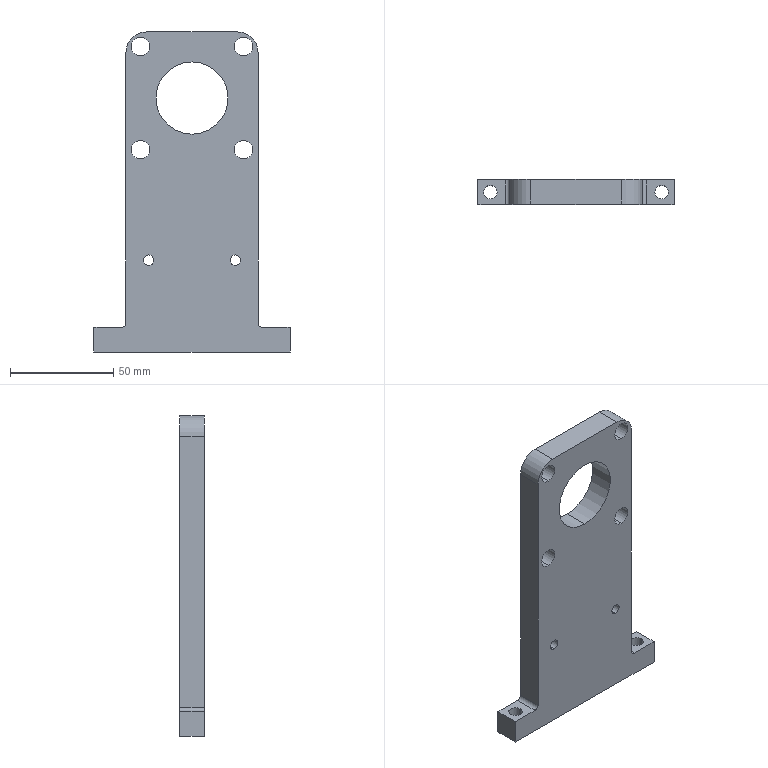Part | 1 solid | 40 faces | box 95 x 12 x 155 mm | volume 106731 mm3 | cylinder 26 | plane 10 | cone 4 | commonest cylinder face diameters 5 x8 9 x8 6.5 x4 4 x2 20 x2 35 x2
STEP:
#1=CARTESIAN_POINT('',(72.5,12.,102.5));
#2=VERTEX_POINT('',#1);
#3=CARTESIAN_POINT('',(72.5,12.,93.5));
#4=VERTEX_POINT('',#3);
#5=CARTESIAN_POINT('',(72.5,12.,98.));
#6=DIRECTION('',(0.,-1.,0.));
#7=DIRECTION('',(0.,0.,-1.));
#8=AXIS2_PLACEMENT_3D('',#5,#6,#7);
#9=CIRCLE('',#8,4.5);
#10=EDGE_CURVE('',#2,#4,#9,.T.);
#11=ORIENTED_EDGE('',*,*,#10,.F.);
#12=CARTESIAN_POINT('',(72.5,0.,102.5));
#13=VERTEX_POINT('',#12);
#14=CARTESIAN_POINT('',(72.5,0.,102.5));
#15=DIRECTION('',(0.,-1.,0.));
#16=VECTOR('',#15,1000.);
#17=LINE('',#14,#16);
#18=EDGE_CURVE('',#2,#13,#17,.T.);
#19=ORIENTED_EDGE('',*,*,#18,.T.);
#20=CARTESIAN_POINT('',(72.5,0.,93.5));
#21=VERTEX_POINT('',#20);
#22=CARTESIAN_POINT('',(72.5,0.,98.));
#23=DIRECTION('',(0.,-1.,0.));
#24=DIRECTION('',(0.,0.,-1.));
#25=AXIS2_PLACEMENT_3D('',#22,#23,#24);
#26=CIRCLE('',#25,4.5);
#27=EDGE_CURVE('',#13,#21,#26,.T.);
#28=ORIENTED_EDGE('',*,*,#27,.T.);
#29=CARTESIAN_POINT('',(72.5,0.,93.5));
#30=DIRECTION('',(0.,-1.,0.));
#31=VECTOR('',#30,1000.);
#32=LINE('',#29,#31);
#33=EDGE_CURVE('',#4,#21,#32,.T.);
#34=ORIENTED_EDGE('',*,*,#33,.F.);
#35=EDGE_LOOP('',(#11,#19,#28,#34));
#36=FACE_OUTER_BOUND('',#35,.T.);
#37=CARTESIAN_POINT('',(72.5,0.,98.));
#38=DIRECTION('',(0.,-1.,0.));
#39=DIRECTION('',(0.,0.,-1.));
#40=AXIS2_PLACEMENT_3D('',#37,#38,#39);
#41=CYLINDRICAL_SURFACE('',#40,4.5);
#42=ADVANCED_FACE('',(#36),#41,.F.);
#43=CARTESIAN_POINT('',(72.5,12.,152.5));
#44=VERTEX_POINT('',#43);
#45=CARTESIAN_POINT('',(72.5,12.,143.5));
#46=VERTEX_POINT('',#45);
#47=CARTESIAN_POINT('',(72.5,12.,148.));
#48=DIRECTION('',(0.,-1.,0.));
#49=DIRECTION('',(0.,0.,-1.));
#50=AXIS2_PLACEMENT_3D('',#47,#48,#49);
#51=CIRCLE('',#50,4.5);
#52=EDGE_CURVE('',#44,#46,#51,.T.);
#53=ORIENTED_EDGE('',*,*,#52,.F.);
#54=CARTESIAN_POINT('',(72.5,0.,152.5));
#55=VERTEX_POINT('',#54);
#56=CARTESIAN_POINT('',(72.5,0.,152.5));
#57=DIRECTION('',(0.,-1.,0.));
#58=VECTOR('',#57,1000.);
#59=LINE('',#56,#58);
#60=EDGE_CURVE('',#44,#55,#59,.T.);
#61=ORIENTED_EDGE('',*,*,#60,.T.);
#62=CARTESIAN_POINT('',(72.5,0.,143.5));
#63=VERTEX_POINT('',#62);
#64=CARTESIAN_POINT('',(72.5,0.,148.));
#65=DIRECTION('',(0.,-1.,0.));
#66=DIRECTION('',(0.,0.,-1.));
#67=AXIS2_PLACEMENT_3D('',#64,#65,#66);
#68=CIRCLE('',#67,4.5);
#69=EDGE_CURVE('',#55,#63,#68,.T.);
#70=ORIENTED_EDGE('',*,*,#69,.T.);
#71=CARTESIAN_POINT('',(72.5,0.,143.5));
#72=DIRECTION('',(0.,-1.,0.));
#73=VECTOR('',#72,1000.);
#74=LINE('',#71,#73);
#75=EDGE_CURVE('',#46,#63,#74,.T.);
#76=ORIENTED_EDGE('',*,*,#75,.F.);
#77=EDGE_LOOP('',(#53,#61,#70,#76));
#78=FACE_OUTER_BOUND('',#77,.T.);
#79=CARTESIAN_POINT('',(72.5,0.,148.));
#80=DIRECTION('',(0.,-1.,0.));
#81=DIRECTION('',(0.,0.,-1.));
#82=AXIS2_PLACEMENT_3D('',#79,#80,#81);
#83=CYLINDRICAL_SURFACE('',#82,4.5);
#84=ADVANCED_FACE('',(#78),#83,.F.);
#85=CARTESIAN_POINT('',(22.5,12.,152.5));
#86=VERTEX_POINT('',#85);
#87=CARTESIAN_POINT('',(22.5,12.,143.5));
#88=VERTEX_POINT('',#87);
#89=CARTESIAN_POINT('',(22.5,12.,148.));
#90=DIRECTION('',(0.,-1.,0.));
#91=DIRECTION('',(0.,0.,-1.));
#92=AXIS2_PLACEMENT_3D('',#89,#90,#91);
#93=CIRCLE('',#92,4.5);
#94=EDGE_CURVE('',#86,#88,#93,.T.);
#95=ORIENTED_EDGE('',*,*,#94,.F.);
#96=CARTESIAN_POINT('',(22.5,0.,152.5));
#97=VERTEX_POINT('',#96);
#98=CARTESIAN_POINT('',(22.5,0.,152.5));
#99=DIRECTION('',(0.,-1.,0.));
#100=VECTOR('',#99,1000.);
#101=LINE('',#98,#100);
#102=EDGE_CURVE('',#86,#97,#101,.T.);
#103=ORIENTED_EDGE('',*,*,#102,.T.);
#104=CARTESIAN_POINT('',(22.5,0.,143.5));
#105=VERTEX_POINT('',#104);
#106=CARTESIAN_POINT('',(22.5,0.,148.));
#107=DIRECTION('',(0.,-1.,0.));
#108=DIRECTION('',(0.,0.,-1.));
#109=AXIS2_PLACEMENT_3D('',#106,#107,#108);
#110=CIRCLE('',#109,4.5);
#111=EDGE_CURVE('',#97,#105,#110,.T.);
#112=ORIENTED_EDGE('',*,*,#111,.T.);
#113=CARTESIAN_POINT('',(22.5,0.,143.5));
#114=DIRECTION('',(0.,-1.,0.));
#115=VECTOR('',#114,1000.);
#116=LINE('',#113,#115);
#117=EDGE_CURVE('',#88,#105,#116,.T.);
#118=ORIENTED_EDGE('',*,*,#117,.F.);
#119=EDGE_LOOP('',(#95,#103,#112,#118));
#120=FACE_OUTER_BOUND('',#119,.T.);
#121=CARTESIAN_POINT('',(22.5,0.,148.));
#122=DIRECTION('',(0.,-1.,0.));
#123=DIRECTION('',(0.,0.,-1.));
#124=AXIS2_PLACEMENT_3D('',#121,#122,#123);
#125=CYLINDRICAL_SURFACE('',#124,4.5);
#126=ADVANCED_FACE('',(#120),#125,.F.);
#127=CARTESIAN_POINT('',(22.5,12.,102.5));
#128=VERTEX_POINT('',#127);
#129=CARTESIAN_POINT('',(22.5,12.,93.5));
#130=VERTEX_POINT('',#129);
#131=CARTESIAN_POINT('',(22.5,12.,98.));
#132=DIRECTION('',(0.,-1.,0.));
#133=DIRECTION('',(0.,0.,-1.));
#134=AXIS2_PLACEMENT_3D('',#131,#132,#133);
#135=CIRCLE('',#134,4.5);
#136=EDGE_CURVE('',#128,#130,#135,.T.);
#137=ORIENTED_EDGE('',*,*,#136,.F.);
#138=CARTESIAN_POINT('',(22.5,0.,102.5));
#139=VERTEX_POINT('',#138);
#140=CARTESIAN_POINT('',(22.5,0.,102.5));
#141=DIRECTION('',(0.,-1.,0.));
#142=VECTOR('',#141,1000.);
#143=LINE('',#140,#142);
#144=EDGE_CURVE('',#128,#139,#143,.T.);
#145=ORIENTED_EDGE('',*,*,#144,.T.);
#146=CARTESIAN_POINT('',(22.5,0.,93.5));
#147=VERTEX_POINT('',#146);
#148=CARTESIAN_POINT('',(22.5,0.,98.));
#149=DIRECTION('',(0.,-1.,0.));
#150=DIRECTION('',(0.,0.,-1.));
#151=AXIS2_PLACEMENT_3D('',#148,#149,#150);
#152=CIRCLE('',#151,4.5);
#153=EDGE_CURVE('',#139,#147,#152,.T.);
#154=ORIENTED_EDGE('',*,*,#153,.T.);
#155=CARTESIAN_POINT('',(22.5,0.,93.5));
#156=DIRECTION('',(0.,-1.,0.));
#157=VECTOR('',#156,1000.);
#158=LINE('',#155,#157);
#159=EDGE_CURVE('',#130,#147,#158,.T.);
#160=ORIENTED_EDGE('',*,*,#159,.F.);
#161=EDGE_LOOP('',(#137,#145,#154,#160));
#162=FACE_OUTER_BOUND('',#161,.T.);
#163=CARTESIAN_POINT('',(22.5,0.,98.));
#164=DIRECTION('',(0.,-1.,0.));
#165=DIRECTION('',(0.,0.,-1.));
#166=AXIS2_PLACEMENT_3D('',#163,#164,#165);
#167=CYLINDRICAL_SURFACE('',#166,4.5);
#168=ADVANCED_FACE('',(#162),#167,.F.);
#169=CARTESIAN_POINT('',(68.5,12.,47.));
#170=VERTEX_POINT('',#169);
#171=CARTESIAN_POINT('',(68.5,12.,42.));
#172=VERTEX_POINT('',#171);
#173=CARTESIAN_POINT('',(68.5,12.,44.5));
#174=DIRECTION('',(0.,-1.,0.));
#175=DIRECTION('',(0.,0.,-1.));
#176=AXIS2_PLACEMENT_3D('',#173,#174,#175);
#177=CIRCLE('',#176,2.5);
#178=EDGE_CURVE('',#170,#172,#177,.T.);
#179=ORIENTED_EDGE('',*,*,#178,.F.);
#180=CARTESIAN_POINT('',(68.5,0.,47.));
#181=VERTEX_POINT('',#180);
#182=CARTESIAN_POINT('',(68.5,0.,47.));
#183=DIRECTION('',(0.,-1.,0.));
#184=VECTOR('',#183,1000.);
#185=LINE('',#182,#184);
#186=EDGE_CURVE('',#170,#181,#185,.T.);
#187=ORIENTED_EDGE('',*,*,#186,.T.);
#188=CARTESIAN_POINT('',(68.5,0.,42.));
#189=VERTEX_POINT('',#188);
#190=CARTESIAN_POINT('',(68.5,0.,44.5));
#191=DIRECTION('',(0.,-1.,0.));
#192=DIRECTION('',(0.,0.,-1.));
#193=AXIS2_PLACEMENT_3D('',#190,#191,#192);
#194=CIRCLE('',#193,2.5);
#195=EDGE_CURVE('',#181,#189,#194,.T.);
#196=ORIENTED_EDGE('',*,*,#195,.T.);
#197=CARTESIAN_POINT('',(68.5,0.,42.));
#198=DIRECTION('',(0.,-1.,0.));
#199=VECTOR('',#198,1000.);
#200=LINE('',#197,#199);
#201=EDGE_CURVE('',#172,#189,#200,.T.);
#202=ORIENTED_EDGE('',*,*,#201,.F.);
#203=EDGE_LOOP('',(#179,#187,#196,#202));
#204=FACE_OUTER_BOUND('',#203,.T.);
#205=CARTESIAN_POINT('',(68.5,0.,44.5));
#206=DIRECTION('',(0.,-1.,0.));
#207=DIRECTION('',(0.,0.,-1.));
#208=AXIS2_PLACEMENT_3D('',#205,#206,#207);
#209=CYLINDRICAL_SURFACE('',#208,2.5);
#210=ADVANCED_FACE('',(#204),#209,.F.);
#211=CARTESIAN_POINT('',(26.5,12.,47.));
#212=VERTEX_POINT('',#211);
#213=CARTESIAN_POINT('',(26.5,12.,42.));
#214=VERTEX_POINT('',#213);
#215=CARTESIAN_POINT('',(26.5,12.,44.5));
#216=DIRECTION('',(0.,-1.,0.));
#217=DIRECTION('',(0.,0.,-1.));
#218=AXIS2_PLACEMENT_3D('',#215,#216,#217);
#219=CIRCLE('',#218,2.5);
#220=EDGE_CURVE('',#212,#214,#219,.T.);
#221=ORIENTED_EDGE('',*,*,#220,.F.);
#222=CARTESIAN_POINT('',(26.5,0.,47.));
#223=VERTEX_POINT('',#222);
#224=CARTESIAN_POINT('',(26.5,0.,47.));
#225=DIRECTION('',(0.,-1.,0.));
#226=VECTOR('',#225,1000.);
#227=LINE('',#224,#226);
#228=EDGE_CURVE('',#212,#223,#227,.T.);
#229=ORIENTED_EDGE('',*,*,#228,.T.);
#230=CARTESIAN_POINT('',(26.5,0.,42.));
#231=VERTEX_POINT('',#230);
#232=CARTESIAN_POINT('',(26.5,0.,44.5));
#233=DIRECTION('',(0.,-1.,0.));
#234=DIRECTION('',(0.,0.,-1.));
#235=AXIS2_PLACEMENT_3D('',#232,#233,#234);
#236=CIRCLE('',#235,2.5);
#237=EDGE_CURVE('',#223,#231,#236,.T.);
#238=ORIENTED_EDGE('',*,*,#237,.T.);
#239=CARTESIAN_POINT('',(26.5,0.,42.));
#240=DIRECTION('',(0.,-1.,0.));
#241=VECTOR('',#240,1000.);
#242=LINE('',#239,#241);
#243=EDGE_CURVE('',#214,#231,#242,.T.);
#244=ORIENTED_EDGE('',*,*,#243,.F.);
#245=EDGE_LOOP('',(#221,#229,#238,#244));
#246=FACE_OUTER_BOUND('',#245,.T.);
#247=CARTESIAN_POINT('',(26.5,0.,44.5));
#248=DIRECTION('',(0.,-1.,0.));
#249=DIRECTION('',(0.,0.,-1.));
#250=AXIS2_PLACEMENT_3D('',#247,#248,#249);
#251=CYLINDRICAL_SURFACE('',#250,2.5);
#252=ADVANCED_FACE('',(#246),#251,.F.);
#253=CARTESIAN_POINT('',(70.,6.,10.));
#254=VERTEX_POINT('',#253);
#255=CARTESIAN_POINT('',(65.,6.,10.));
#256=VERTEX_POINT('',#255);
#257=CARTESIAN_POINT('',(67.5,6.,10.));
#258=DIRECTION('',(0.,0.,-1.));
#259=DIRECTION('',(-1.,0.,0.));
#260=AXIS2_PLACEMENT_3D('',#257,#258,#259);
#261=CIRCLE('',#260,2.5);
#262=EDGE_CURVE('',#254,#256,#261,.T.);
#263=ORIENTED_EDGE('',*,*,#262,.F.);
#264=CARTESIAN_POINT('',(70.,6.,0.));
#265=VERTEX_POINT('',#264);
#266=CARTESIAN_POINT('',(70.,6.,0.));
#267=DIRECTION('',(0.,0.,-1.));
#268=VECTOR('',#267,1000.);
#269=LINE('',#266,#268);
#270=EDGE_CURVE('',#254,#265,#269,.T.);
#271=ORIENTED_EDGE('',*,*,#270,.T.);
#272=CARTESIAN_POINT('',(65.,6.,0.));
#273=VERTEX_POINT('',#272);
#274=CARTESIAN_POINT('',(67.5,6.,0.));
#275=DIRECTION('',(0.,0.,-1.));
#276=DIRECTION('',(-1.,0.,0.));
#277=AXIS2_PLACEMENT_3D('',#274,#275,#276);
#278=CIRCLE('',#277,2.5);
#279=EDGE_CURVE('',#265,#273,#278,.T.);
#280=ORIENTED_EDGE('',*,*,#279,.T.);
#281=CARTESIAN_POINT('',(65.,6.,0.));
#282=DIRECTION('',(0.,0.,-1.));
#283=VECTOR('',#282,1000.);
#284=LINE('',#281,#283);
#285=EDGE_CURVE('',#256,#273,#284,.T.);
#286=ORIENTED_EDGE('',*,*,#285,.F.);
#287=EDGE_LOOP('',(#263,#271,#280,#286));
#288=FACE_OUTER_BOUND('',#287,.T.);
#289=CARTESIAN_POINT('',(67.5,6.,0.));
#290=DIRECTION('',(0.,0.,-1.));
#291=DIRECTION('',(-1.,0.,0.));
#292=AXIS2_PLACEMENT_3D('',#289,#290,#291);
#293=CYLINDRICAL_SURFACE('',#292,2.5);
#294=ADVANCED_FACE('',(#288),#293,.F.);
#295=CARTESIAN_POINT('',(67.5,6.,11.502));
#296=VERTEX_POINT('',#295);
#297=CARTESIAN_POINT('',(65.,6.,10.));
#298=DIRECTION('',(-0.8572,0.,-0.515));
#299=VECTOR('',#298,1000.);
#300=LINE('',#297,#299);
#301=EDGE_CURVE('',#296,#256,#300,.T.);
#302=ORIENTED_EDGE('',*,*,#301,.F.);
#303=CARTESIAN_POINT('',(70.,6.,10.));
#304=DIRECTION('',(0.8572,0.,-0.515));
#305=VECTOR('',#304,1000.);
#306=LINE('',#303,#305);
#307=EDGE_CURVE('',#296,#254,#306,.T.);
#308=ORIENTED_EDGE('',*,*,#307,.T.);
#309=ORIENTED_EDGE('',*,*,#262,.T.);
#310=EDGE_LOOP('',(#302,#308,#309));
#311=FACE_OUTER_BOUND('',#310,.T.);
#312=CARTESIAN_POINT('',(67.5,6.,10.));
#313=DIRECTION('',(0.,0.,-1.));
#314=DIRECTION('',(-1.,0.,0.));
#315=AXIS2_PLACEMENT_3D('',#312,#313,#314);
#316=CONICAL_SURFACE('',#315,2.5,1.03);
#317=ADVANCED_FACE('',(#311),#316,.F.);
#318=CARTESIAN_POINT('',(30.,6.,10.));
#319=VERTEX_POINT('',#318);
#320=CARTESIAN_POINT('',(25.,6.,10.));
#321=VERTEX_POINT('',#320);
#322=CARTESIAN_POINT('',(27.5,6.,10.));
#323=DIRECTION('',(0.,0.,-1.));
#324=DIRECTION('',(-1.,0.,0.));
#325=AXIS2_PLACEMENT_3D('',#322,#323,#324);
#326=CIRCLE('',#325,2.5);
#327=EDGE_CURVE('',#319,#321,#326,.T.);
#328=ORIENTED_EDGE('',*,*,#327,.F.);
#329=CARTESIAN_POINT('',(30.,6.,0.));
#330=VERTEX_POINT('',#329);
#331=CARTESIAN_POINT('',(30.,6.,0.));
#332=DIRECTION('',(0.,0.,-1.));
#333=VECTOR('',#332,1000.);
#334=LINE('',#331,#333);
#335=EDGE_CURVE('',#319,#330,#334,.T.);
#336=ORIENTED_EDGE('',*,*,#335,.T.);
#337=CARTESIAN_POINT('',(25.,6.,0.));
#338=VERTEX_POINT('',#337);
#339=CARTESIAN_POINT('',(27.5,6.,0.));
#340=DIRECTION('',(0.,0.,-1.));
#341=DIRECTION('',(-1.,0.,0.));
#342=AXIS2_PLACEMENT_3D('',#339,#340,#341);
#343=CIRCLE('',#342,2.5);
#344=EDGE_CURVE('',#330,#338,#343,.T.);
#345=ORIENTED_EDGE('',*,*,#344,.T.);
#346=CARTESIAN_POINT('',(25.,6.,0.));
#347=DIRECTION('',(0.,0.,-1.));
#348=VECTOR('',#347,1000.);
#349=LINE('',#346,#348);
#350=EDGE_CURVE('',#321,#338,#349,.T.);
#351=ORIENTED_EDGE('',*,*,#350,.F.);
#352=EDGE_LOOP('',(#328,#336,#345,#351));
#353=FACE_OUTER_BOUND('',#352,.T.);
#354=CARTESIAN_POINT('',(27.5,6.,0.));
#355=DIRECTION('',(0.,0.,-1.));
#356=DIRECTION('',(-1.,0.,0.));
#357=AXIS2_PLACEMENT_3D('',#354,#355,#356);
#358=CYLINDRICAL_SURFACE('',#357,2.5);
#359=ADVANCED_FACE('',(#353),#358,.F.);
#360=CARTESIAN_POINT('',(27.5,6.,11.502));
#361=VERTEX_POINT('',#360);
#362=CARTESIAN_POINT('',(25.,6.,10.));
#363=DIRECTION('',(-0.8572,0.,-0.515));
#364=VECTOR('',#363,1000.);
#365=LINE('',#362,#364);
#366=EDGE_CURVE('',#361,#321,#365,.T.);
#367=ORIENTED_EDGE('',*,*,#366,.F.);
#368=CARTESIAN_POINT('',(30.,6.,10.));
#369=DIRECTION('',(0.8572,0.,-0.515));
#370=VECTOR('',#369,1000.);
#371=LINE('',#368,#370);
#372=EDGE_CURVE('',#361,#319,#371,.T.);
#373=ORIENTED_EDGE('',*,*,#372,.T.);
#374=ORIENTED_EDGE('',*,*,#327,.T.);
#375=EDGE_LOOP('',(#367,#373,#374));
#376=FACE_OUTER_BOUND('',#375,.T.);
#377=CARTESIAN_POINT('',(27.5,6.,10.));
#378=DIRECTION('',(0.,0.,-1.));
#379=DIRECTION('',(-1.,0.,0.));
#380=AXIS2_PLACEMENT_3D('',#377,#378,#379);
#381=CONICAL_SURFACE('',#380,2.5,1.03);
#382=ADVANCED_FACE('',(#376),#381,.F.);
#383=CARTESIAN_POINT('',(47.5,0.,105.5));
#384=VERTEX_POINT('',#383);
#385=CARTESIAN_POINT('',(47.5,0.,140.5));
#386=VERTEX_POINT('',#385);
#387=CARTESIAN_POINT('',(47.5,0.,123.));
#388=DIRECTION('',(0.,1.,0.));
#389=DIRECTION('',(0.,0.,1.));
#390=AXIS2_PLACEMENT_3D('',#387,#388,#389);
#391=CIRCLE('',#390,17.5);
#392=EDGE_CURVE('',#384,#386,#391,.T.);
#393=ORIENTED_EDGE('',*,*,#392,.F.);
#394=CARTESIAN_POINT('',(47.5,12.,105.5));
#395=VERTEX_POINT('',#394);
#396=CARTESIAN_POINT('',(47.5,0.,105.5));
#397=DIRECTION('',(0.,1.,0.));
#398=VECTOR('',#397,1000.);
#399=LINE('',#396,#398);
#400=EDGE_CURVE('',#384,#395,#399,.T.);
#401=ORIENTED_EDGE('',*,*,#400,.T.);
#402=CARTESIAN_POINT('',(47.5,12.,140.5));
#403=VERTEX_POINT('',#402);
#404=CARTESIAN_POINT('',(47.5,12.,123.));
#405=DIRECTION('',(0.,1.,0.));
#406=DIRECTION('',(0.,0.,1.));
#407=AXIS2_PLACEMENT_3D('',#404,#405,#406);
#408=CIRCLE('',#407,17.5);
#409=EDGE_CURVE('',#395,#403,#408,.T.);
#410=ORIENTED_EDGE('',*,*,#409,.T.);
#411=CARTESIAN_POINT('',(47.5,0.,140.5));
#412=DIRECTION('',(0.,1.,0.));
#413=VECTOR('',#412,1000.);
#414=LINE('',#411,#413);
#415=EDGE_CURVE('',#386,#403,#414,.T.);
#416=ORIENTED_EDGE('',*,*,#415,.F.);
#417=EDGE_LOOP('',(#393,#401,#410,#416));
#418=FACE_OUTER_BOUND('',#417,.T.);
#419=CARTESIAN_POINT('',(47.5,0.,123.));
#420=DIRECTION('',(0.,1.,0.));
#421=DIRECTION('',(0.,0.,1.));
#422=AXIS2_PLACEMENT_3D('',#419,#420,#421);
#423=CYLINDRICAL_SURFACE('',#422,17.5);
#424=ADVANCED_FACE('',(#418),#423,.F.);
#425=CARTESIAN_POINT('',(2.75,6.,0.));
#426=VERTEX_POINT('',#425);
#427=CARTESIAN_POINT('',(9.25,6.,0.));
#428=VERTEX_POINT('',#427);
#429=CARTESIAN_POINT('',(6.,6.,0.));
#430=DIRECTION('',(0.,0.,1.));
#431=DIRECTION('',(1.,0.,0.));
#432=AXIS2_PLACEMENT_3D('',#429,#430,#431);
#433=CIRCLE('',#432,3.25);
#434=EDGE_CURVE('',#426,#428,#433,.T.);
#435=ORIENTED_EDGE('',*,*,#434,.F.);
#436=CARTESIAN_POINT('',(2.75,6.,12.));
#437=VERTEX_POINT('',#436);
#438=CARTESIAN_POINT('',(2.75,6.,12.));
#439=DIRECTION('',(0.,0.,1.));
#440=VECTOR('',#439,1000.);
#441=LINE('',#438,#440);
#442=EDGE_CURVE('',#426,#437,#441,.T.);
#443=ORIENTED_EDGE('',*,*,#442,.T.);
#444=CARTESIAN_POINT('',(9.25,6.,12.));
#445=VERTEX_POINT('',#444);
#446=CARTESIAN_POINT('',(6.,6.,12.));
#447=DIRECTION('',(0.,0.,1.));
#448=DIRECTION('',(1.,0.,0.));
#449=AXIS2_PLACEMENT_3D('',#446,#447,#448);
#450=CIRCLE('',#449,3.25);
#451=EDGE_CURVE('',#437,#445,#450,.T.);
#452=ORIENTED_EDGE('',*,*,#451,.T.);
#453=CARTESIAN_POINT('',(9.25,6.,12.));
#454=DIRECTION('',(0.,0.,1.));
#455=VECTOR('',#454,1000.);
#456=LINE('',#453,#455);
#457=EDGE_CURVE('',#428,#445,#456,.T.);
#458=ORIENTED_EDGE('',*,*,#457,.F.);
#459=EDGE_LOOP('',(#435,#443,#452,#458));
#460=FACE_OUTER_BOUND('',#459,.T.);
#461=CARTESIAN_POINT('',(6.,6.,12.));
#462=DIRECTION('',(0.,0.,1.));
#463=DIRECTION('',(1.,0.,0.));
#464=AXIS2_PLACEMENT_3D('',#461,#462,#463);
#465=CYLINDRICAL_SURFACE('',#464,3.25);
#466=ADVANCED_FACE('',(#460),#465,.F.);
#467=CARTESIAN_POINT('',(85.75,6.,0.));
#468=VERTEX_POINT('',#467);
#469=CARTESIAN_POINT('',(92.25,6.,0.));
#470=VERTEX_POINT('',#469);
#471=CARTESIAN_POINT('',(89.,6.,0.));
#472=DIRECTION('',(0.,0.,1.));
#473=DIRECTION('',(1.,0.,0.));
#474=AXIS2_PLACEMENT_3D('',#471,#472,#473);
#475=CIRCLE('',#474,3.25);
#476=EDGE_CURVE('',#468,#470,#475,.T.);
#477=ORIENTED_EDGE('',*,*,#476,.F.);
#478=CARTESIAN_POINT('',(85.75,6.,12.));
#479=VERTEX_POINT('',#478);
#480=CARTESIAN_POINT('',(85.75,6.,12.));
#481=DIRECTION('',(0.,0.,1.));
#482=VECTOR('',#481,1000.);
#483=LINE('',#480,#482);
#484=EDGE_CURVE('',#468,#479,#483,.T.);
#485=ORIENTED_EDGE('',*,*,#484,.T.);
#486=CARTESIAN_POINT('',(92.25,6.,12.));
#487=VERTEX_POINT('',#486);
#488=CARTESIAN_POINT('',(89.,6.,12.));
#489=DIRECTION('',(0.,0.,1.));
#490=DIRECTION('',(1.,0.,0.));
#491=AXIS2_PLACEMENT_3D('',#488,#489,#490);
#492=CIRCLE('',#491,3.25);
#493=EDGE_CURVE('',#479,#487,#492,.T.);
#494=ORIENTED_EDGE('',*,*,#493,.T.);
#495=CARTESIAN_POINT('',(92.25,6.,12.));
#496=DIRECTION('',(0.,0.,1.));
#497=VECTOR('',#496,1000.);
#498=LINE('',#495,#497);
#499=EDGE_CURVE('',#470,#487,#498,.T.);
#500=ORIENTED_EDGE('',*,*,#499,.F.);
#501=EDGE_LOOP('',(#477,#485,#494,#500));
#502=FACE_OUTER_BOUND('',#501,.T.);
#503=CARTESIAN_POINT('',(89.,6.,12.));
#504=DIRECTION('',(0.,0.,1.));
#505=DIRECTION('',(1.,0.,0.));
#506=AXIS2_PLACEMENT_3D('',#503,#504,#505);
#507=CYLINDRICAL_SURFACE('',#506,3.25);
#508=ADVANCED_FACE('',(#502),#507,.F.);
#509=CARTESIAN_POINT('',(0.,0.,0.));
#510=VERTEX_POINT('',#509);
#511=CARTESIAN_POINT('',(0.,0.,12.));
#512=VERTEX_POINT('',#511);
#513=CARTESIAN_POINT('',(0.,0.,155.));
#514=DIRECTION('',(0.,0.,1.));
#515=VECTOR('',#514,1000.);
#516=LINE('',#513,#515);
#517=EDGE_CURVE('',#510,#512,#516,.T.);
#518=ORIENTED_EDGE('',*,*,#517,.T.);
#519=CARTESIAN_POINT('',(0.,12.,12.));
#520=VERTEX_POINT('',#519);
#521=CARTESIAN_POINT('',(0.,0.,12.));
#522=DIRECTION('',(0.,1.,0.));
#523=VECTOR('',#522,1000.);
#524=LINE('',#521,#523);
#525=EDGE_CURVE('',#512,#520,#524,.T.);
#526=ORIENTED_EDGE('',*,*,#525,.T.);
#527=CARTESIAN_POINT('',(0.,12.,0.));
#528=VERTEX_POINT('',#527);
#529=CARTESIAN_POINT('',(0.,12.,155.));
#530=DIRECTION('',(0.,0.,1.));
#531=VECTOR('',#530,1000.);
#532=LINE('',#529,#531);
#533=EDGE_CURVE('',#528,#520,#532,.T.);
#534=ORIENTED_EDGE('',*,*,#533,.F.);
#535=CARTESIAN_POINT('',(0.,12.,0.));
#536=DIRECTION('',(0.,-1.,0.));
#537=VECTOR('',#536,1000.);
#538=LINE('',#535,#537);
#539=EDGE_CURVE('',#528,#510,#538,.T.);
#540=ORIENTED_EDGE('',*,*,#539,.T.);
#541=EDGE_LOOP('',(#518,#526,#534,#540));
#542=FACE_OUTER_BOUND('',#541,.T.);
#543=CARTESIAN_POINT('',(0.,12.,155.));
#544=DIRECTION('',(1.,0.,0.));
#545=DIRECTION('',(0.,0.,-1.));
#546=AXIS2_PLACEMENT_3D('',#543,#544,#545);
#547=PLANE('',#546);
#548=ADVANCED_FACE('',(#542),#547,.F.);
#549=CARTESIAN_POINT('',(25.5,12.,155.));
#550=VERTEX_POINT('',#549);
#551=CARTESIAN_POINT('',(69.5,12.,155.));
#552=VERTEX_POINT('',#551);
#553=CARTESIAN_POINT('',(95.,12.,155.));
#554=DIRECTION('',(1.,0.,0.));
#555=VECTOR('',#554,1000.);
#556=LINE('',#553,#555);
#557=EDGE_CURVE('',#550,#552,#556,.T.);
#558=ORIENTED_EDGE('',*,*,#557,.F.);
#559=CARTESIAN_POINT('',(25.5,0.,155.));
#560=VERTEX_POINT('',#559);
#561=CARTESIAN_POINT('',(25.5,12.,155.));
#562=DIRECTION('',(0.,-1.,0.));
#563=VECTOR('',#562,1000.);
#564=LINE('',#561,#563);
#565=EDGE_CURVE('',#550,#560,#564,.T.);
#566=ORIENTED_EDGE('',*,*,#565,.T.);
#567=CARTESIAN_POINT('',(69.5,0.,155.));
#568=VERTEX_POINT('',#567);
#569=CARTESIAN_POINT('',(95.,0.,155.));
#570=DIRECTION('',(1.,0.,0.));
#571=VECTOR('',#570,1000.);
#572=LINE('',#569,#571);
#573=EDGE_CURVE('',#560,#568,#572,.T.);
#574=ORIENTED_EDGE('',*,*,#573,.T.);
#575=CARTESIAN_POINT('',(69.5,12.,155.));
#576=DIRECTION('',(0.,1.,0.));
#577=VECTOR('',#576,1000.);
#578=LINE('',#575,#577);
#579=EDGE_CURVE('',#568,#552,#578,.T.);
#580=ORIENTED_EDGE('',*,*,#579,.T.);
#581=EDGE_LOOP('',(#558,#566,#574,#580));
#582=FACE_OUTER_BOUND('',#581,.T.);
#583=CARTESIAN_POINT('',(95.,12.,155.));
#584=DIRECTION('',(0.,0.,-1.));
#585=DIRECTION('',(-1.,0.,0.));
#586=AXIS2_PLACEMENT_3D('',#583,#584,#585);
#587=PLANE('',#586);
#588=ADVANCED_FACE('',(#582),#587,.F.);
#589=CARTESIAN_POINT('',(95.,12.,12.));
#590=VERTEX_POINT('',#589);
#591=CARTESIAN_POINT('',(95.,12.,0.));
#592=VERTEX_POINT('',#591);
#593=CARTESIAN_POINT('',(95.,12.,0.));
#594=DIRECTION('',(0.,0.,-1.));
#595=VECTOR('',#594,1000.);
#596=LINE('',#593,#595);
#597=EDGE_CURVE('',#590,#592,#596,.T.);
#598=ORIENTED_EDGE('',*,*,#597,.F.);
#599=CARTESIAN_POINT('',(95.,0.,12.));
#600=VERTEX_POINT('',#599);
#601=CARTESIAN_POINT('',(95.,0.,12.));
#602=DIRECTION('',(0.,1.,0.));
#603=VECTOR('',#602,1000.);
#604=LINE('',#601,#603);
#605=EDGE_CURVE('',#600,#590,#604,.T.);
#606=ORIENTED_EDGE('',*,*,#605,.F.);
#607=CARTESIAN_POINT('',(95.,0.,0.));
#608=VERTEX_POINT('',#607);
#609=CARTESIAN_POINT('',(95.,0.,0.));
#610=DIRECTION('',(0.,0.,-1.));
#611=VECTOR('',#610,1000.);
#612=LINE('',#609,#611);
#613=EDGE_CURVE('',#600,#608,#612,.T.);
#614=ORIENTED_EDGE('',*,*,#613,.T.);
#615=CARTESIAN_POINT('',(95.,12.,0.));
#616=DIRECTION('',(0.,-1.,0.));
#617=VECTOR('',#616,1000.);
#618=LINE('',#615,#617);
#619=EDGE_CURVE('',#592,#608,#618,.T.);
#620=ORIENTED_EDGE('',*,*,#619,.F.);
#621=EDGE_LOOP('',(#598,#606,#614,#620));
#622=FACE_OUTER_BOUND('',#621,.T.);
#623=CARTESIAN_POINT('',(95.,12.,0.));
#624=DIRECTION('',(-1.,0.,0.));
#625=DIRECTION('',(0.,0.,1.));
#626=AXIS2_PLACEMENT_3D('',#623,#624,#625);
#627=PLANE('',#626);
#628=ADVANCED_FACE('',(#622),#627,.F.);
#629=CARTESIAN_POINT('',(67.5,6.,0.));
#630=DIRECTION('',(0.,0.,-1.));
#631=DIRECTION('',(-1.,0.,0.));
#632=AXIS2_PLACEMENT_3D('',#629,#630,#631);
#633=CIRCLE('',#632,2.5);
#634=EDGE_CURVE('',#273,#265,#633,.T.);
#635=ORIENTED_EDGE('',*,*,#634,.F.);
#636=ORIENTED_EDGE('',*,*,#279,.F.);
#637=EDGE_LOOP('',(#635,#636));
#638=FACE_BOUND('',#637,.T.);
#639=CARTESIAN_POINT('',(27.5,6.,0.));
#640=DIRECTION('',(0.,0.,-1.));
#641=DIRECTION('',(-1.,0.,0.));
#642=AXIS2_PLACEMENT_3D('',#639,#640,#641);
#643=CIRCLE('',#642,2.5);
#644=EDGE_CURVE('',#338,#330,#643,.T.);
#645=ORIENTED_EDGE('',*,*,#644,.F.);
#646=ORIENTED_EDGE('',*,*,#344,.F.);
#647=EDGE_LOOP('',(#645,#646));
#648=FACE_BOUND('',#647,.T.);
#649=CARTESIAN_POINT('',(6.,6.,0.));
#650=DIRECTION('',(0.,0.,1.));
#651=DIRECTION('',(1.,0.,0.));
#652=AXIS2_PLACEMENT_3D('',#649,#650,#651);
#653=CIRCLE('',#652,3.25);
#654=EDGE_CURVE('',#428,#426,#653,.T.);
#655=ORIENTED_EDGE('',*,*,#654,.T.);
#656=ORIENTED_EDGE('',*,*,#434,.T.);
#657=EDGE_LOOP('',(#655,#656));
#658=FACE_BOUND('',#657,.T.);
#659=CARTESIAN_POINT('',(89.,6.,0.));
#660=DIRECTION('',(0.,0.,1.));
#661=DIRECTION('',(1.,0.,0.));
#662=AXIS2_PLACEMENT_3D('',#659,#660,#661);
#663=CIRCLE('',#662,3.25);
#664=EDGE_CURVE('',#470,#468,#663,.T.);
#665=ORIENTED_EDGE('',*,*,#664,.T.);
#666=ORIENTED_EDGE('',*,*,#476,.T.);
#667=EDGE_LOOP('',(#665,#666));
#668=FACE_BOUND('',#667,.T.);
#669=CARTESIAN_POINT('',(0.,0.,0.));
#670=DIRECTION('',(-1.,0.,0.));
#671=VECTOR('',#670,1000.);
#672=LINE('',#669,#671);
#673=EDGE_CURVE('',#608,#510,#672,.T.);
#674=ORIENTED_EDGE('',*,*,#673,.T.);
#675=ORIENTED_EDGE('',*,*,#539,.F.);
#676=CARTESIAN_POINT('',(0.,12.,0.));
#677=DIRECTION('',(-1.,0.,0.));
#678=VECTOR('',#677,1000.);
#679=LINE('',#676,#678);
#680=EDGE_CURVE('',#592,#528,#679,.T.);
#681=ORIENTED_EDGE('',*,*,#680,.F.);
#682=ORIENTED_EDGE('',*,*,#619,.T.);
#683=EDGE_LOOP('',(#674,#675,#681,#682));
#684=FACE_OUTER_BOUND('',#683,.T.);
#685=CARTESIAN_POINT('',(0.,12.,0.));
#686=DIRECTION('',(0.,0.,1.));
#687=DIRECTION('',(1.,0.,0.));
#688=AXIS2_PLACEMENT_3D('',#685,#686,#687);
#689=PLANE('',#688);
#690=ADVANCED_FACE('',(#638,#648,#658,#668,#684),#689,.F.);
#691=CARTESIAN_POINT('',(72.5,12.,98.));
#692=DIRECTION('',(0.,-1.,0.));
#693=DIRECTION('',(0.,0.,-1.));
#694=AXIS2_PLACEMENT_3D('',#691,#692,#693);
#695=CIRCLE('',#694,4.5);
#696=EDGE_CURVE('',#4,#2,#695,.T.);
#697=ORIENTED_EDGE('',*,*,#696,.T.);
#698=ORIENTED_EDGE('',*,*,#10,.T.);
#699=EDGE_LOOP('',(#697,#698));
#700=FACE_BOUND('',#699,.T.);
#701=CARTESIAN_POINT('',(72.5,12.,148.));
#702=DIRECTION('',(0.,-1.,0.));
#703=DIRECTION('',(0.,0.,-1.));
#704=AXIS2_PLACEMENT_3D('',#701,#702,#703);
#705=CIRCLE('',#704,4.5);
#706=EDGE_CURVE('',#46,#44,#705,.T.);
#707=ORIENTED_EDGE('',*,*,#706,.T.);
#708=ORIENTED_EDGE('',*,*,#52,.T.);
#709=EDGE_LOOP('',(#707,#708));
#710=FACE_BOUND('',#709,.T.);
#711=CARTESIAN_POINT('',(22.5,12.,148.));
#712=DIRECTION('',(0.,-1.,0.));
#713=DIRECTION('',(0.,0.,-1.));
#714=AXIS2_PLACEMENT_3D('',#711,#712,#713);
#715=CIRCLE('',#714,4.5);
#716=EDGE_CURVE('',#88,#86,#715,.T.);
#717=ORIENTED_EDGE('',*,*,#716,.T.);
#718=ORIENTED_EDGE('',*,*,#94,.T.);
#719=EDGE_LOOP('',(#717,#718));
#720=FACE_BOUND('',#719,.T.);
#721=CARTESIAN_POINT('',(22.5,12.,98.));
#722=DIRECTION('',(0.,-1.,0.));
#723=DIRECTION('',(0.,0.,-1.));
#724=AXIS2_PLACEMENT_3D('',#721,#722,#723);
#725=CIRCLE('',#724,4.5);
#726=EDGE_CURVE('',#130,#128,#725,.T.);
#727=ORIENTED_EDGE('',*,*,#726,.T.);
#728=ORIENTED_EDGE('',*,*,#136,.T.);
#729=EDGE_LOOP('',(#727,#728));
#730=FACE_BOUND('',#729,.T.);
#731=CARTESIAN_POINT('',(68.5,12.,44.5));
#732=DIRECTION('',(0.,-1.,0.));
#733=DIRECTION('',(0.,0.,-1.));
#734=AXIS2_PLACEMENT_3D('',#731,#732,#733);
#735=CIRCLE('',#734,2.5);
#736=EDGE_CURVE('',#172,#170,#735,.T.);
#737=ORIENTED_EDGE('',*,*,#736,.T.);
#738=ORIENTED_EDGE('',*,*,#178,.T.);
#739=EDGE_LOOP('',(#737,#738));
#740=FACE_BOUND('',#739,.T.);
#741=CARTESIAN_POINT('',(26.5,12.,44.5));
#742=DIRECTION('',(0.,-1.,0.));
#743=DIRECTION('',(0.,0.,-1.));
#744=AXIS2_PLACEMENT_3D('',#741,#742,#743);
#745=CIRCLE('',#744,2.5);
#746=EDGE_CURVE('',#214,#212,#745,.T.);
#747=ORIENTED_EDGE('',*,*,#746,.T.);
#748=ORIENTED_EDGE('',*,*,#220,.T.);
#749=EDGE_LOOP('',(#747,#748));
#750=FACE_BOUND('',#749,.T.);
#751=CARTESIAN_POINT('',(47.5,12.,123.));
#752=DIRECTION('',(0.,1.,0.));
#753=DIRECTION('',(0.,0.,1.));
#754=AXIS2_PLACEMENT_3D('',#751,#752,#753);
#755=CIRCLE('',#754,17.5);
#756=EDGE_CURVE('',#403,#395,#755,.T.);
#757=ORIENTED_EDGE('',*,*,#756,.F.);
#758=ORIENTED_EDGE('',*,*,#409,.F.);
#759=EDGE_LOOP('',(#757,#758));
#760=FACE_BOUND('',#759,.T.);
#761=CARTESIAN_POINT('',(15.5,12.,145.));
#762=VERTEX_POINT('',#761);
#763=CARTESIAN_POINT('',(15.5,12.,14.));
#764=VERTEX_POINT('',#763);
#765=CARTESIAN_POINT('',(15.5,12.,155.));
#766=DIRECTION('',(0.,0.,-1.));
#767=VECTOR('',#766,1000.);
#768=LINE('',#765,#767);
#769=EDGE_CURVE('',#762,#764,#768,.T.);
#770=ORIENTED_EDGE('',*,*,#769,.F.);
#771=CARTESIAN_POINT('',(25.5,12.,145.));
#772=DIRECTION('',(0.,1.,0.));
#773=DIRECTION('',(0.,0.,-1.));
#774=AXIS2_PLACEMENT_3D('',#771,#772,#773);
#775=CIRCLE('',#774,10.);
#776=EDGE_CURVE('',#762,#550,#775,.T.);
#777=ORIENTED_EDGE('',*,*,#776,.T.);
#778=ORIENTED_EDGE('',*,*,#557,.T.);
#779=CARTESIAN_POINT('',(79.5,12.,145.));
#780=VERTEX_POINT('',#779);
#781=CARTESIAN_POINT('',(69.5,12.,145.));
#782=DIRECTION('',(0.,1.,0.));
#783=DIRECTION('',(0.,0.,-1.));
#784=AXIS2_PLACEMENT_3D('',#781,#782,#783);
#785=CIRCLE('',#784,10.);
#786=EDGE_CURVE('',#552,#780,#785,.T.);
#787=ORIENTED_EDGE('',*,*,#786,.T.);
#788=CARTESIAN_POINT('',(79.5,12.,14.));
#789=VERTEX_POINT('',#788);
#790=CARTESIAN_POINT('',(79.5,12.,155.));
#791=DIRECTION('',(0.,0.,1.));
#792=VECTOR('',#791,1000.);
#793=LINE('',#790,#792);
#794=EDGE_CURVE('',#789,#780,#793,.T.);
#795=ORIENTED_EDGE('',*,*,#794,.F.);
#796=CARTESIAN_POINT('',(81.5,12.,12.));
#797=VERTEX_POINT('',#796);
#798=CARTESIAN_POINT('',(81.5,12.,14.));
#799=DIRECTION('',(0.,-1.,0.));
#800=DIRECTION('',(0.,0.,-1.));
#801=AXIS2_PLACEMENT_3D('',#798,#799,#800);
#802=CIRCLE('',#801,2.);
#803=EDGE_CURVE('',#789,#797,#802,.T.);
#804=ORIENTED_EDGE('',*,*,#803,.T.);
#805=CARTESIAN_POINT('',(95.,12.,12.));
#806=DIRECTION('',(-1.,0.,0.));
#807=VECTOR('',#806,1000.);
#808=LINE('',#805,#807);
#809=EDGE_CURVE('',#590,#797,#808,.T.);
#810=ORIENTED_EDGE('',*,*,#809,.F.);
#811=ORIENTED_EDGE('',*,*,#597,.T.);
#812=ORIENTED_EDGE('',*,*,#680,.T.);
#813=ORIENTED_EDGE('',*,*,#533,.T.);
#814=CARTESIAN_POINT('',(13.5,12.,12.));
#815=VERTEX_POINT('',#814);
#816=CARTESIAN_POINT('',(0.,12.,12.));
#817=DIRECTION('',(-1.,0.,0.));
#818=VECTOR('',#817,1000.);
#819=LINE('',#816,#818);
#820=EDGE_CURVE('',#815,#520,#819,.T.);
#821=ORIENTED_EDGE('',*,*,#820,.F.);
#822=CARTESIAN_POINT('',(13.5,12.,14.));
#823=DIRECTION('',(0.,-1.,0.));
#824=DIRECTION('',(0.,0.,-1.));
#825=AXIS2_PLACEMENT_3D('',#822,#823,#824);
#826=CIRCLE('',#825,2.);
#827=EDGE_CURVE('',#815,#764,#826,.T.);
#828=ORIENTED_EDGE('',*,*,#827,.T.);
#829=EDGE_LOOP('',(#770,#777,#778,#787,#795,#804,#810,#811,#812,#813,#821,#828));
#830=FACE_OUTER_BOUND('',#829,.T.);
#831=CARTESIAN_POINT('',(0.,12.,0.));
#832=DIRECTION('',(0.,-1.,0.));
#833=DIRECTION('',(0.,0.,-1.));
#834=AXIS2_PLACEMENT_3D('',#831,#832,#833);
#835=PLANE('',#834);
#836=ADVANCED_FACE('',(#700,#710,#720,#730,#740,#750,#760,#830),#835,.F.);
#837=CARTESIAN_POINT('',(72.5,0.,98.));
#838=DIRECTION('',(0.,-1.,0.));
#839=DIRECTION('',(0.,0.,-1.));
#840=AXIS2_PLACEMENT_3D('',#837,#838,#839);
#841=CIRCLE('',#840,4.5);
#842=EDGE_CURVE('',#21,#13,#841,.T.);
#843=ORIENTED_EDGE('',*,*,#842,.F.);
#844=ORIENTED_EDGE('',*,*,#27,.F.);
#845=EDGE_LOOP('',(#843,#844));
#846=FACE_BOUND('',#845,.T.);
#847=CARTESIAN_POINT('',(72.5,0.,148.));
#848=DIRECTION('',(0.,-1.,0.));
#849=DIRECTION('',(0.,0.,-1.));
#850=AXIS2_PLACEMENT_3D('',#847,#848,#849);
#851=CIRCLE('',#850,4.5);
#852=EDGE_CURVE('',#63,#55,#851,.T.);
#853=ORIENTED_EDGE('',*,*,#852,.F.);
#854=ORIENTED_EDGE('',*,*,#69,.F.);
#855=EDGE_LOOP('',(#853,#854));
#856=FACE_BOUND('',#855,.T.);
#857=CARTESIAN_POINT('',(22.5,0.,148.));
#858=DIRECTION('',(0.,-1.,0.));
#859=DIRECTION('',(0.,0.,-1.));
#860=AXIS2_PLACEMENT_3D('',#857,#858,#859);
#861=CIRCLE('',#860,4.5);
#862=EDGE_CURVE('',#105,#97,#861,.T.);
#863=ORIENTED_EDGE('',*,*,#862,.F.);
#864=ORIENTED_EDGE('',*,*,#111,.F.);
#865=EDGE_LOOP('',(#863,#864));
#866=FACE_BOUND('',#865,.T.);
#867=CARTESIAN_POINT('',(22.5,0.,98.));
#868=DIRECTION('',(0.,-1.,0.));
#869=DIRECTION('',(0.,0.,-1.));
#870=AXIS2_PLACEMENT_3D('',#867,#868,#869);
#871=CIRCLE('',#870,4.5);
#872=EDGE_CURVE('',#147,#139,#871,.T.);
#873=ORIENTED_EDGE('',*,*,#872,.F.);
#874=ORIENTED_EDGE('',*,*,#153,.F.);
#875=EDGE_LOOP('',(#873,#874));
#876=FACE_BOUND('',#875,.T.);
#877=CARTESIAN_POINT('',(68.5,0.,44.5));
#878=DIRECTION('',(0.,-1.,0.));
#879=DIRECTION('',(0.,0.,-1.));
#880=AXIS2_PLACEMENT_3D('',#877,#878,#879);
#881=CIRCLE('',#880,2.5);
#882=EDGE_CURVE('',#189,#181,#881,.T.);
#883=ORIENTED_EDGE('',*,*,#882,.F.);
#884=ORIENTED_EDGE('',*,*,#195,.F.);
#885=EDGE_LOOP('',(#883,#884));
#886=FACE_BOUND('',#885,.T.);
#887=CARTESIAN_POINT('',(26.5,0.,44.5));
#888=DIRECTION('',(0.,-1.,0.));
#889=DIRECTION('',(0.,0.,-1.));
#890=AXIS2_PLACEMENT_3D('',#887,#888,#889);
#891=CIRCLE('',#890,2.5);
#892=EDGE_CURVE('',#231,#223,#891,.T.);
#893=ORIENTED_EDGE('',*,*,#892,.F.);
#894=ORIENTED_EDGE('',*,*,#237,.F.);
#895=EDGE_LOOP('',(#893,#894));
#896=FACE_BOUND('',#895,.T.);
#897=CARTESIAN_POINT('',(47.5,0.,123.));
#898=DIRECTION('',(0.,1.,0.));
#899=DIRECTION('',(0.,0.,1.));
#900=AXIS2_PLACEMENT_3D('',#897,#898,#899);
#901=CIRCLE('',#900,17.5);
#902=EDGE_CURVE('',#386,#384,#901,.T.);
#903=ORIENTED_EDGE('',*,*,#902,.T.);
#904=ORIENTED_EDGE('',*,*,#392,.T.);
#905=EDGE_LOOP('',(#903,#904));
#906=FACE_BOUND('',#905,.T.);
#907=ORIENTED_EDGE('',*,*,#573,.F.);
#908=CARTESIAN_POINT('',(15.5,0.,145.));
#909=VERTEX_POINT('',#908);
#910=CARTESIAN_POINT('',(25.5,0.,145.));
#911=DIRECTION('',(0.,-1.,0.));
#912=DIRECTION('',(0.,0.,-1.));
#913=AXIS2_PLACEMENT_3D('',#910,#911,#912);
#914=CIRCLE('',#913,10.);
#915=EDGE_CURVE('',#560,#909,#914,.T.);
#916=ORIENTED_EDGE('',*,*,#915,.T.);
#917=CARTESIAN_POINT('',(15.5,0.,14.));
#918=VERTEX_POINT('',#917);
#919=CARTESIAN_POINT('',(15.5,0.,155.));
#920=DIRECTION('',(0.,0.,-1.));
#921=VECTOR('',#920,1000.);
#922=LINE('',#919,#921);
#923=EDGE_CURVE('',#909,#918,#922,.T.);
#924=ORIENTED_EDGE('',*,*,#923,.T.);
#925=CARTESIAN_POINT('',(13.5,0.,12.));
#926=VERTEX_POINT('',#925);
#927=CARTESIAN_POINT('',(13.5,0.,14.));
#928=DIRECTION('',(0.,1.,0.));
#929=DIRECTION('',(0.,0.,-1.));
#930=AXIS2_PLACEMENT_3D('',#927,#928,#929);
#931=CIRCLE('',#930,2.);
#932=EDGE_CURVE('',#918,#926,#931,.T.);
#933=ORIENTED_EDGE('',*,*,#932,.T.);
#934=CARTESIAN_POINT('',(0.,0.,12.));
#935=DIRECTION('',(-1.,0.,0.));
#936=VECTOR('',#935,1000.);
#937=LINE('',#934,#936);
#938=EDGE_CURVE('',#926,#512,#937,.T.);
#939=ORIENTED_EDGE('',*,*,#938,.T.);
#940=ORIENTED_EDGE('',*,*,#517,.F.);
#941=ORIENTED_EDGE('',*,*,#673,.F.);
#942=ORIENTED_EDGE('',*,*,#613,.F.);
#943=CARTESIAN_POINT('',(81.5,0.,12.));
#944=VERTEX_POINT('',#943);
#945=CARTESIAN_POINT('',(95.,0.,12.));
#946=DIRECTION('',(-1.,0.,0.));
#947=VECTOR('',#946,1000.);
#948=LINE('',#945,#947);
#949=EDGE_CURVE('',#600,#944,#948,.T.);
#950=ORIENTED_EDGE('',*,*,#949,.T.);
#951=CARTESIAN_POINT('',(79.5,0.,14.));
#952=VERTEX_POINT('',#951);
#953=CARTESIAN_POINT('',(81.5,0.,14.));
#954=DIRECTION('',(0.,1.,0.));
#955=DIRECTION('',(0.,0.,-1.));
#956=AXIS2_PLACEMENT_3D('',#953,#954,#955);
#957=CIRCLE('',#956,2.);
#958=EDGE_CURVE('',#944,#952,#957,.T.);
#959=ORIENTED_EDGE('',*,*,#958,.T.);
#960=CARTESIAN_POINT('',(79.5,0.,145.));
#961=VERTEX_POINT('',#960);
#962=CARTESIAN_POINT('',(79.5,0.,155.));
#963=DIRECTION('',(0.,0.,1.));
#964=VECTOR('',#963,1000.);
#965=LINE('',#962,#964);
#966=EDGE_CURVE('',#952,#961,#965,.T.);
#967=ORIENTED_EDGE('',*,*,#966,.T.);
#968=CARTESIAN_POINT('',(69.5,0.,145.));
#969=DIRECTION('',(0.,-1.,0.));
#970=DIRECTION('',(0.,0.,-1.));
#971=AXIS2_PLACEMENT_3D('',#968,#969,#970);
#972=CIRCLE('',#971,10.);
#973=EDGE_CURVE('',#961,#568,#972,.T.);
#974=ORIENTED_EDGE('',*,*,#973,.T.);
#975=EDGE_LOOP('',(#907,#916,#924,#933,#939,#940,#941,#942,#950,#959,#967,#974));
#976=FACE_OUTER_BOUND('',#975,.T.);
#977=CARTESIAN_POINT('',(0.,0.,0.));
#978=DIRECTION('',(0.,-1.,0.));
#979=DIRECTION('',(0.,0.,-1.));
#980=AXIS2_PLACEMENT_3D('',#977,#978,#979);
#981=PLANE('',#980);
#982=ADVANCED_FACE('',(#846,#856,#866,#876,#886,#896,#906,#976),#981,.T.);
#983=CARTESIAN_POINT('',(6.,6.,12.));
#984=DIRECTION('',(0.,0.,1.));
#985=DIRECTION('',(1.,0.,0.));
#986=AXIS2_PLACEMENT_3D('',#983,#984,#985);
#987=CIRCLE('',#986,3.25);
#988=EDGE_CURVE('',#445,#437,#987,.T.);
#989=ORIENTED_EDGE('',*,*,#988,.F.);
#990=ORIENTED_EDGE('',*,*,#451,.F.);
#991=EDGE_LOOP('',(#989,#990));
#992=FACE_BOUND('',#991,.T.);
#993=ORIENTED_EDGE('',*,*,#938,.F.);
#994=CARTESIAN_POINT('',(13.5,12.,12.));
#995=DIRECTION('',(0.,1.,0.));
#996=VECTOR('',#995,1000.);
#997=LINE('',#994,#996);
#998=EDGE_CURVE('',#926,#815,#997,.T.);
#999=ORIENTED_EDGE('',*,*,#998,.T.);
#1000=ORIENTED_EDGE('',*,*,#820,.T.);
#1001=ORIENTED_EDGE('',*,*,#525,.F.);
#1002=EDGE_LOOP('',(#993,#999,#1000,#1001));
#1003=FACE_OUTER_BOUND('',#1002,.T.);
#1004=CARTESIAN_POINT('',(0.,0.,12.));
#1005=DIRECTION('',(0.,0.,-1.));
#1006=DIRECTION('',(-1.,0.,0.));
#1007=AXIS2_PLACEMENT_3D('',#1004,#1005,#1006);
#1008=PLANE('',#1007);
#1009=ADVANCED_FACE('',(#992,#1003),#1008,.F.);
#1010=ORIENTED_EDGE('',*,*,#769,.T.);
#1011=CARTESIAN_POINT('',(15.5,0.,14.));
#1012=DIRECTION('',(0.,-1.,0.));
#1013=VECTOR('',#1012,1000.);
#1014=LINE('',#1011,#1013);
#1015=EDGE_CURVE('',#764,#918,#1014,.T.);
#1016=ORIENTED_EDGE('',*,*,#1015,.T.);
#1017=ORIENTED_EDGE('',*,*,#923,.F.);
#1018=CARTESIAN_POINT('',(15.5,0.,145.));
#1019=DIRECTION('',(0.,1.,0.));
#1020=VECTOR('',#1019,1000.);
#1021=LINE('',#1018,#1020);
#1022=EDGE_CURVE('',#909,#762,#1021,.T.);
#1023=ORIENTED_EDGE('',*,*,#1022,.T.);
#1024=EDGE_LOOP('',(#1010,#1016,#1017,#1023));
#1025=FACE_OUTER_BOUND('',#1024,.T.);
#1026=CARTESIAN_POINT('',(15.5,0.,155.));
#1027=DIRECTION('',(1.,0.,0.));
#1028=DIRECTION('',(0.,0.,-1.));
#1029=AXIS2_PLACEMENT_3D('',#1026,#1027,#1028);
#1030=PLANE('',#1029);
#1031=ADVANCED_FACE('',(#1025),#1030,.F.);
#1032=ORIENTED_EDGE('',*,*,#966,.F.);
#1033=CARTESIAN_POINT('',(79.5,12.,14.));
#1034=DIRECTION('',(0.,1.,0.));
#1035=VECTOR('',#1034,1000.);
#1036=LINE('',#1033,#1035);
#1037=EDGE_CURVE('',#952,#789,#1036,.T.);
#1038=ORIENTED_EDGE('',*,*,#1037,.T.);
#1039=ORIENTED_EDGE('',*,*,#794,.T.);
#1040=CARTESIAN_POINT('',(79.5,0.,145.));
#1041=DIRECTION('',(0.,-1.,0.));
#1042=VECTOR('',#1041,1000.);
#1043=LINE('',#1040,#1042);
#1044=EDGE_CURVE('',#780,#961,#1043,.T.);
#1045=ORIENTED_EDGE('',*,*,#1044,.T.);
#1046=EDGE_LOOP('',(#1032,#1038,#1039,#1045));
#1047=FACE_OUTER_BOUND('',#1046,.T.);
#1048=CARTESIAN_POINT('',(79.5,0.,155.));
#1049=DIRECTION('',(-1.,0.,0.));
#1050=DIRECTION('',(0.,0.,1.));
#1051=AXIS2_PLACEMENT_3D('',#1048,#1049,#1050);
#1052=PLANE('',#1051);
#1053=ADVANCED_FACE('',(#1047),#1052,.F.);
#1054=CARTESIAN_POINT('',(89.,6.,12.));
#1055=DIRECTION('',(0.,0.,1.));
#1056=DIRECTION('',(1.,0.,0.));
#1057=AXIS2_PLACEMENT_3D('',#1054,#1055,#1056);
#1058=CIRCLE('',#1057,3.25);
#1059=EDGE_CURVE('',#487,#479,#1058,.T.);
#1060=ORIENTED_EDGE('',*,*,#1059,.F.);
#1061=ORIENTED_EDGE('',*,*,#493,.F.);
#1062=EDGE_LOOP('',(#1060,#1061));
#1063=FACE_BOUND('',#1062,.T.);
#1064=ORIENTED_EDGE('',*,*,#809,.T.);
#1065=CARTESIAN_POINT('',(81.5,0.,12.));
#1066=DIRECTION('',(0.,-1.,0.));
#1067=VECTOR('',#1066,1000.);
#1068=LINE('',#1065,#1067);
#1069=EDGE_CURVE('',#797,#944,#1068,.T.);
#1070=ORIENTED_EDGE('',*,*,#1069,.T.);
#1071=ORIENTED_EDGE('',*,*,#949,.F.);
#1072=ORIENTED_EDGE('',*,*,#605,.T.);
#1073=EDGE_LOOP('',(#1064,#1070,#1071,#1072));
#1074=FACE_OUTER_BOUND('',#1073,.T.);
#1075=CARTESIAN_POINT('',(95.,0.,12.));
#1076=DIRECTION('',(0.,0.,-1.));
#1077=DIRECTION('',(-1.,0.,0.));
#1078=AXIS2_PLACEMENT_3D('',#1075,#1076,#1077);
#1079=PLANE('',#1078);
#1080=ADVANCED_FACE('',(#1063,#1074),#1079,.F.);
#1081=ORIENTED_EDGE('',*,*,#484,.F.);
#1082=ORIENTED_EDGE('',*,*,#664,.F.);
#1083=ORIENTED_EDGE('',*,*,#499,.T.);
#1084=ORIENTED_EDGE('',*,*,#1059,.T.);
#1085=EDGE_LOOP('',(#1081,#1082,#1083,#1084));
#1086=FACE_OUTER_BOUND('',#1085,.T.);
#1087=CARTESIAN_POINT('',(89.,6.,12.));
#1088=DIRECTION('',(0.,0.,1.));
#1089=DIRECTION('',(1.,0.,0.));
#1090=AXIS2_PLACEMENT_3D('',#1087,#1088,#1089);
#1091=CYLINDRICAL_SURFACE('',#1090,3.25);
#1092=ADVANCED_FACE('',(#1086),#1091,.F.);
#1093=ORIENTED_EDGE('',*,*,#442,.F.);
#1094=ORIENTED_EDGE('',*,*,#654,.F.);
#1095=ORIENTED_EDGE('',*,*,#457,.T.);
#1096=ORIENTED_EDGE('',*,*,#988,.T.);
#1097=EDGE_LOOP('',(#1093,#1094,#1095,#1096));
#1098=FACE_OUTER_BOUND('',#1097,.T.);
#1099=CARTESIAN_POINT('',(6.,6.,12.));
#1100=DIRECTION('',(0.,0.,1.));
#1101=DIRECTION('',(1.,0.,0.));
#1102=AXIS2_PLACEMENT_3D('',#1099,#1100,#1101);
#1103=CYLINDRICAL_SURFACE('',#1102,3.25);
#1104=ADVANCED_FACE('',(#1098),#1103,.F.);
#1105=ORIENTED_EDGE('',*,*,#400,.F.);
#1106=ORIENTED_EDGE('',*,*,#902,.F.);
#1107=ORIENTED_EDGE('',*,*,#415,.T.);
#1108=ORIENTED_EDGE('',*,*,#756,.T.);
#1109=EDGE_LOOP('',(#1105,#1106,#1107,#1108));
#1110=FACE_OUTER_BOUND('',#1109,.T.);
#1111=CARTESIAN_POINT('',(47.5,0.,123.));
#1112=DIRECTION('',(0.,1.,0.));
#1113=DIRECTION('',(0.,0.,1.));
#1114=AXIS2_PLACEMENT_3D('',#1111,#1112,#1113);
#1115=CYLINDRICAL_SURFACE('',#1114,17.5);
#1116=ADVANCED_FACE('',(#1110),#1115,.F.);
#1117=ORIENTED_EDGE('',*,*,#915,.F.);
#1118=ORIENTED_EDGE('',*,*,#565,.F.);
#1119=ORIENTED_EDGE('',*,*,#776,.F.);
#1120=ORIENTED_EDGE('',*,*,#1022,.F.);
#1121=EDGE_LOOP('',(#1117,#1118,#1119,#1120));
#1122=FACE_OUTER_BOUND('',#1121,.T.);
#1123=CARTESIAN_POINT('',(25.5,0.,145.));
#1124=DIRECTION('',(0.,1.,0.));
#1125=DIRECTION('',(0.,0.,1.));
#1126=AXIS2_PLACEMENT_3D('',#1123,#1124,#1125);
#1127=CYLINDRICAL_SURFACE('',#1126,10.);
#1128=ADVANCED_FACE('',(#1122),#1127,.T.);
#1129=ORIENTED_EDGE('',*,*,#973,.F.);
#1130=ORIENTED_EDGE('',*,*,#1044,.F.);
#1131=ORIENTED_EDGE('',*,*,#786,.F.);
#1132=ORIENTED_EDGE('',*,*,#579,.F.);
#1133=EDGE_LOOP('',(#1129,#1130,#1131,#1132));
#1134=FACE_OUTER_BOUND('',#1133,.T.);
#1135=CARTESIAN_POINT('',(69.5,12.,145.));
#1136=DIRECTION('',(0.,1.,0.));
#1137=DIRECTION('',(0.,0.,1.));
#1138=AXIS2_PLACEMENT_3D('',#1135,#1136,#1137);
#1139=CYLINDRICAL_SURFACE('',#1138,10.);
#1140=ADVANCED_FACE('',(#1134),#1139,.T.);
#1141=ORIENTED_EDGE('',*,*,#372,.F.);
#1142=ORIENTED_EDGE('',*,*,#366,.T.);
#1143=CARTESIAN_POINT('',(27.5,6.,10.));
#1144=DIRECTION('',(0.,0.,-1.));
#1145=DIRECTION('',(-1.,0.,0.));
#1146=AXIS2_PLACEMENT_3D('',#1143,#1144,#1145);
#1147=CIRCLE('',#1146,2.5);
#1148=EDGE_CURVE('',#321,#319,#1147,.T.);
#1149=ORIENTED_EDGE('',*,*,#1148,.T.);
#1150=EDGE_LOOP('',(#1141,#1142,#1149));
#1151=FACE_OUTER_BOUND('',#1150,.T.);
#1152=CARTESIAN_POINT('',(27.5,6.,10.));
#1153=DIRECTION('',(0.,0.,-1.));
#1154=DIRECTION('',(-1.,0.,0.));
#1155=AXIS2_PLACEMENT_3D('',#1152,#1153,#1154);
#1156=CONICAL_SURFACE('',#1155,2.5,1.03);
#1157=ADVANCED_FACE('',(#1151),#1156,.F.);
#1158=ORIENTED_EDGE('',*,*,#335,.F.);
#1159=ORIENTED_EDGE('',*,*,#1148,.F.);
#1160=ORIENTED_EDGE('',*,*,#350,.T.);
#1161=ORIENTED_EDGE('',*,*,#644,.T.);
#1162=EDGE_LOOP('',(#1158,#1159,#1160,#1161));
#1163=FACE_OUTER_BOUND('',#1162,.T.);
#1164=CARTESIAN_POINT('',(27.5,6.,0.));
#1165=DIRECTION('',(0.,0.,-1.));
#1166=DIRECTION('',(-1.,0.,0.));
#1167=AXIS2_PLACEMENT_3D('',#1164,#1165,#1166);
#1168=CYLINDRICAL_SURFACE('',#1167,2.5);
#1169=ADVANCED_FACE('',(#1163),#1168,.F.);
#1170=ORIENTED_EDGE('',*,*,#307,.F.);
#1171=ORIENTED_EDGE('',*,*,#301,.T.);
#1172=CARTESIAN_POINT('',(67.5,6.,10.));
#1173=DIRECTION('',(0.,0.,-1.));
#1174=DIRECTION('',(-1.,0.,0.));
#1175=AXIS2_PLACEMENT_3D('',#1172,#1173,#1174);
#1176=CIRCLE('',#1175,2.5);
#1177=EDGE_CURVE('',#256,#254,#1176,.T.);
#1178=ORIENTED_EDGE('',*,*,#1177,.T.);
#1179=EDGE_LOOP('',(#1170,#1171,#1178));
#1180=FACE_OUTER_BOUND('',#1179,.T.);
#1181=CARTESIAN_POINT('',(67.5,6.,10.));
#1182=DIRECTION('',(0.,0.,-1.));
#1183=DIRECTION('',(-1.,0.,0.));
#1184=AXIS2_PLACEMENT_3D('',#1181,#1182,#1183);
#1185=CONICAL_SURFACE('',#1184,2.5,1.03);
#1186=ADVANCED_FACE('',(#1180),#1185,.F.);
#1187=ORIENTED_EDGE('',*,*,#270,.F.);
#1188=ORIENTED_EDGE('',*,*,#1177,.F.);
#1189=ORIENTED_EDGE('',*,*,#285,.T.);
#1190=ORIENTED_EDGE('',*,*,#634,.T.);
#1191=EDGE_LOOP('',(#1187,#1188,#1189,#1190));
#1192=FACE_OUTER_BOUND('',#1191,.T.);
#1193=CARTESIAN_POINT('',(67.5,6.,0.));
#1194=DIRECTION('',(0.,0.,-1.));
#1195=DIRECTION('',(-1.,0.,0.));
#1196=AXIS2_PLACEMENT_3D('',#1193,#1194,#1195);
#1197=CYLINDRICAL_SURFACE('',#1196,2.5);
#1198=ADVANCED_FACE('',(#1192),#1197,.F.);
#1199=ORIENTED_EDGE('',*,*,#932,.F.);
#1200=ORIENTED_EDGE('',*,*,#1015,.F.);
#1201=ORIENTED_EDGE('',*,*,#827,.F.);
#1202=ORIENTED_EDGE('',*,*,#998,.F.);
#1203=EDGE_LOOP('',(#1199,#1200,#1201,#1202));
#1204=FACE_OUTER_BOUND('',#1203,.T.);
#1205=CARTESIAN_POINT('',(13.5,0.,14.));
#1206=DIRECTION('',(0.,-1.,0.));
#1207=DIRECTION('',(0.,0.,-1.));
#1208=AXIS2_PLACEMENT_3D('',#1205,#1206,#1207);
#1209=CYLINDRICAL_SURFACE('',#1208,2.);
#1210=ADVANCED_FACE('',(#1204),#1209,.F.);
#1211=ORIENTED_EDGE('',*,*,#958,.F.);
#1212=ORIENTED_EDGE('',*,*,#1069,.F.);
#1213=ORIENTED_EDGE('',*,*,#803,.F.);
#1214=ORIENTED_EDGE('',*,*,#1037,.F.);
#1215=EDGE_LOOP('',(#1211,#1212,#1213,#1214));
#1216=FACE_OUTER_BOUND('',#1215,.T.);
#1217=CARTESIAN_POINT('',(81.5,0.,14.));
#1218=DIRECTION('',(0.,-1.,0.));
#1219=DIRECTION('',(0.,0.,-1.));
#1220=AXIS2_PLACEMENT_3D('',#1217,#1218,#1219);
#1221=CYLINDRICAL_SURFACE('',#1220,2.);
#1222=ADVANCED_FACE('',(#1216),#1221,.F.);
#1223=ORIENTED_EDGE('',*,*,#228,.F.);
#1224=ORIENTED_EDGE('',*,*,#746,.F.);
#1225=ORIENTED_EDGE('',*,*,#243,.T.);
#1226=ORIENTED_EDGE('',*,*,#892,.T.);
#1227=EDGE_LOOP('',(#1223,#1224,#1225,#1226));
#1228=FACE_OUTER_BOUND('',#1227,.T.);
#1229=CARTESIAN_POINT('',(26.5,0.,44.5));
#1230=DIRECTION('',(0.,-1.,0.));
#1231=DIRECTION('',(0.,0.,-1.));
#1232=AXIS2_PLACEMENT_3D('',#1229,#1230,#1231);
#1233=CYLINDRICAL_SURFACE('',#1232,2.5);
#1234=ADVANCED_FACE('',(#1228),#1233,.F.);
#1235=ORIENTED_EDGE('',*,*,#186,.F.);
#1236=ORIENTED_EDGE('',*,*,#736,.F.);
#1237=ORIENTED_EDGE('',*,*,#201,.T.);
#1238=ORIENTED_EDGE('',*,*,#882,.T.);
#1239=EDGE_LOOP('',(#1235,#1236,#1237,#1238));
#1240=FACE_OUTER_BOUND('',#1239,.T.);
#1241=CARTESIAN_POINT('',(68.5,0.,44.5));
#1242=DIRECTION('',(0.,-1.,0.));
#1243=DIRECTION('',(0.,0.,-1.));
#1244=AXIS2_PLACEMENT_3D('',#1241,#1242,#1243);
#1245=CYLINDRICAL_SURFACE('',#1244,2.5);
#1246=ADVANCED_FACE('',(#1240),#1245,.F.);
#1247=ORIENTED_EDGE('',*,*,#144,.F.);
#1248=ORIENTED_EDGE('',*,*,#726,.F.);
#1249=ORIENTED_EDGE('',*,*,#159,.T.);
#1250=ORIENTED_EDGE('',*,*,#872,.T.);
#1251=EDGE_LOOP('',(#1247,#1248,#1249,#1250));
#1252=FACE_OUTER_BOUND('',#1251,.T.);
#1253=CARTESIAN_POINT('',(22.5,0.,98.));
#1254=DIRECTION('',(0.,-1.,0.));
#1255=DIRECTION('',(0.,0.,-1.));
#1256=AXIS2_PLACEMENT_3D('',#1253,#1254,#1255);
#1257=CYLINDRICAL_SURFACE('',#1256,4.5);
#1258=ADVANCED_FACE('',(#1252),#1257,.F.);
#1259=ORIENTED_EDGE('',*,*,#102,.F.);
#1260=ORIENTED_EDGE('',*,*,#716,.F.);
#1261=ORIENTED_EDGE('',*,*,#117,.T.);
#1262=ORIENTED_EDGE('',*,*,#862,.T.);
#1263=EDGE_LOOP('',(#1259,#1260,#1261,#1262));
#1264=FACE_OUTER_BOUND('',#1263,.T.);
#1265=CARTESIAN_POINT('',(22.5,0.,148.));
#1266=DIRECTION('',(0.,-1.,0.));
#1267=DIRECTION('',(0.,0.,-1.));
#1268=AXIS2_PLACEMENT_3D('',#1265,#1266,#1267);
#1269=CYLINDRICAL_SURFACE('',#1268,4.5);
#1270=ADVANCED_FACE('',(#1264),#1269,.F.);
#1271=ORIENTED_EDGE('',*,*,#60,.F.);
#1272=ORIENTED_EDGE('',*,*,#706,.F.);
#1273=ORIENTED_EDGE('',*,*,#75,.T.);
#1274=ORIENTED_EDGE('',*,*,#852,.T.);
#1275=EDGE_LOOP('',(#1271,#1272,#1273,#1274));
#1276=FACE_OUTER_BOUND('',#1275,.T.);
#1277=CARTESIAN_POINT('',(72.5,0.,148.));
#1278=DIRECTION('',(0.,-1.,0.));
#1279=DIRECTION('',(0.,0.,-1.));
#1280=AXIS2_PLACEMENT_3D('',#1277,#1278,#1279);
#1281=CYLINDRICAL_SURFACE('',#1280,4.5);
#1282=ADVANCED_FACE('',(#1276),#1281,.F.);
#1283=ORIENTED_EDGE('',*,*,#18,.F.);
#1284=ORIENTED_EDGE('',*,*,#696,.F.);
#1285=ORIENTED_EDGE('',*,*,#33,.T.);
#1286=ORIENTED_EDGE('',*,*,#842,.T.);
#1287=EDGE_LOOP('',(#1283,#1284,#1285,#1286));
#1288=FACE_OUTER_BOUND('',#1287,.T.);
#1289=CARTESIAN_POINT('',(72.5,0.,98.));
#1290=DIRECTION('',(0.,-1.,0.));
#1291=DIRECTION('',(0.,0.,-1.));
#1292=AXIS2_PLACEMENT_3D('',#1289,#1290,#1291);
#1293=CYLINDRICAL_SURFACE('',#1292,4.5);
#1294=ADVANCED_FACE('',(#1288),#1293,.F.);
#1295=CLOSED_SHELL('',(#42,#84,#126,#168,#210,#252,#294,#317,#359,#382,#424,#466,#508,#548,#588,#628,#690,#836,#982,#1009,#1031,#1053,#1080,#1092,#1104,#1116,#1128,#1140,#1157,#1169,#1186,#1198,#1210,#1222,#1234,#1246,#1258,#1270,#1282,#1294));
#1296=MANIFOLD_SOLID_BREP('',#1295);
#1297=CARTESIAN_POINT('',(0.,0.,0.));
#1298=DIRECTION('',(0.,0.,1.));
#1299=DIRECTION('',(1.,0.,0.));
#1300=AXIS2_PLACEMENT_3D('',#1297,#1298,#1299);
#1301=(LENGTH_UNIT()NAMED_UNIT(*)SI_UNIT(.MILLI.,.METRE.));
#1302=UNCERTAINTY_MEASURE_WITH_UNIT(LENGTH_MEASURE(0.00001),#1301,'','');
#1303=(NAMED_UNIT(*)PLANE_ANGLE_UNIT()SI_UNIT($,.RADIAN.));
#1304=(NAMED_UNIT(*)SI_UNIT($,.STERADIAN.)SOLID_ANGLE_UNIT());
#1305=(GEOMETRIC_REPRESENTATION_CONTEXT(3)GLOBAL_UNCERTAINTY_ASSIGNED_CONTEXT((#1302))GLOBAL_UNIT_ASSIGNED_CONTEXT((#1301,#1303,#1304))REPRESENTATION_CONTEXT('',''));
#1306=ADVANCED_BREP_SHAPE_REPRESENTATION('',(#1296,#1300),#1305);